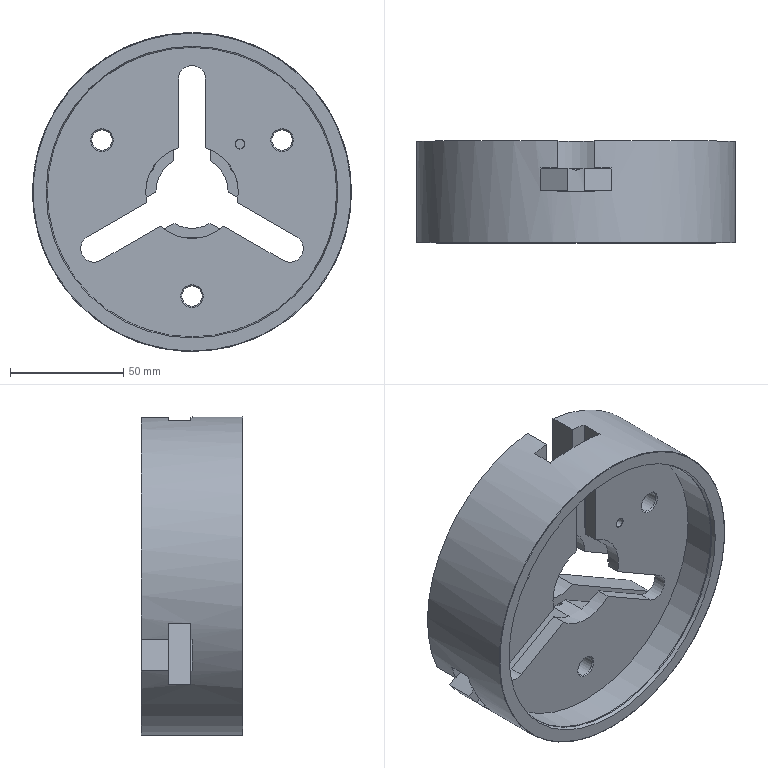NC program | NX | posted with a generic post | part box 141 x 45 x 141 mm
Whole program:
N10 G17 G21 G94 G90
(PLANAR_MILL_1 , TOOL : D12)
N12 T06 M6
N14 G54
N16 G17 G0 G90 X0. Y0. S0 M3
N18 G43 Z100. H6
N20 Z-27.5
N22 G94 G1 Z-30.5 F250.
N24 Y50.
N26 G0 Z100.
(PLANAR_MILL_1_COPY , TOOL : D12)
N28 Y0.
N30 Z-27.5
N32 G1 Z-30.5
N34 X-43.301 Y-25.
N36 G0 Z100.
(PLANAR_MILL_1_COPY_1 , TOOL : D12)
N38 X0. Y0.
N40 Z-27.5
N42 G1 Z-30.5
N44 X43.301 Y-25.
N46 G0 Z100.
N48 M5
N50 M2